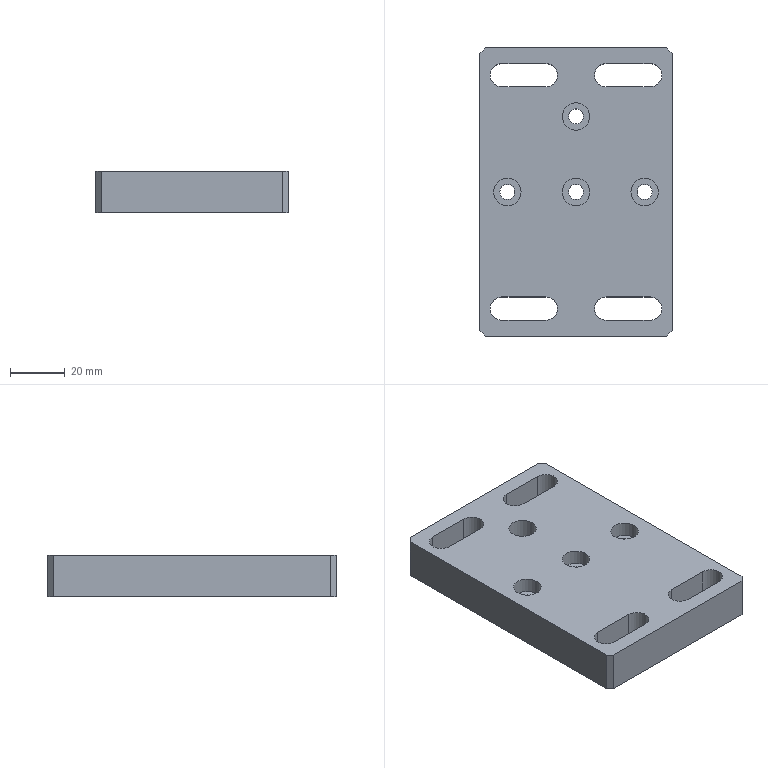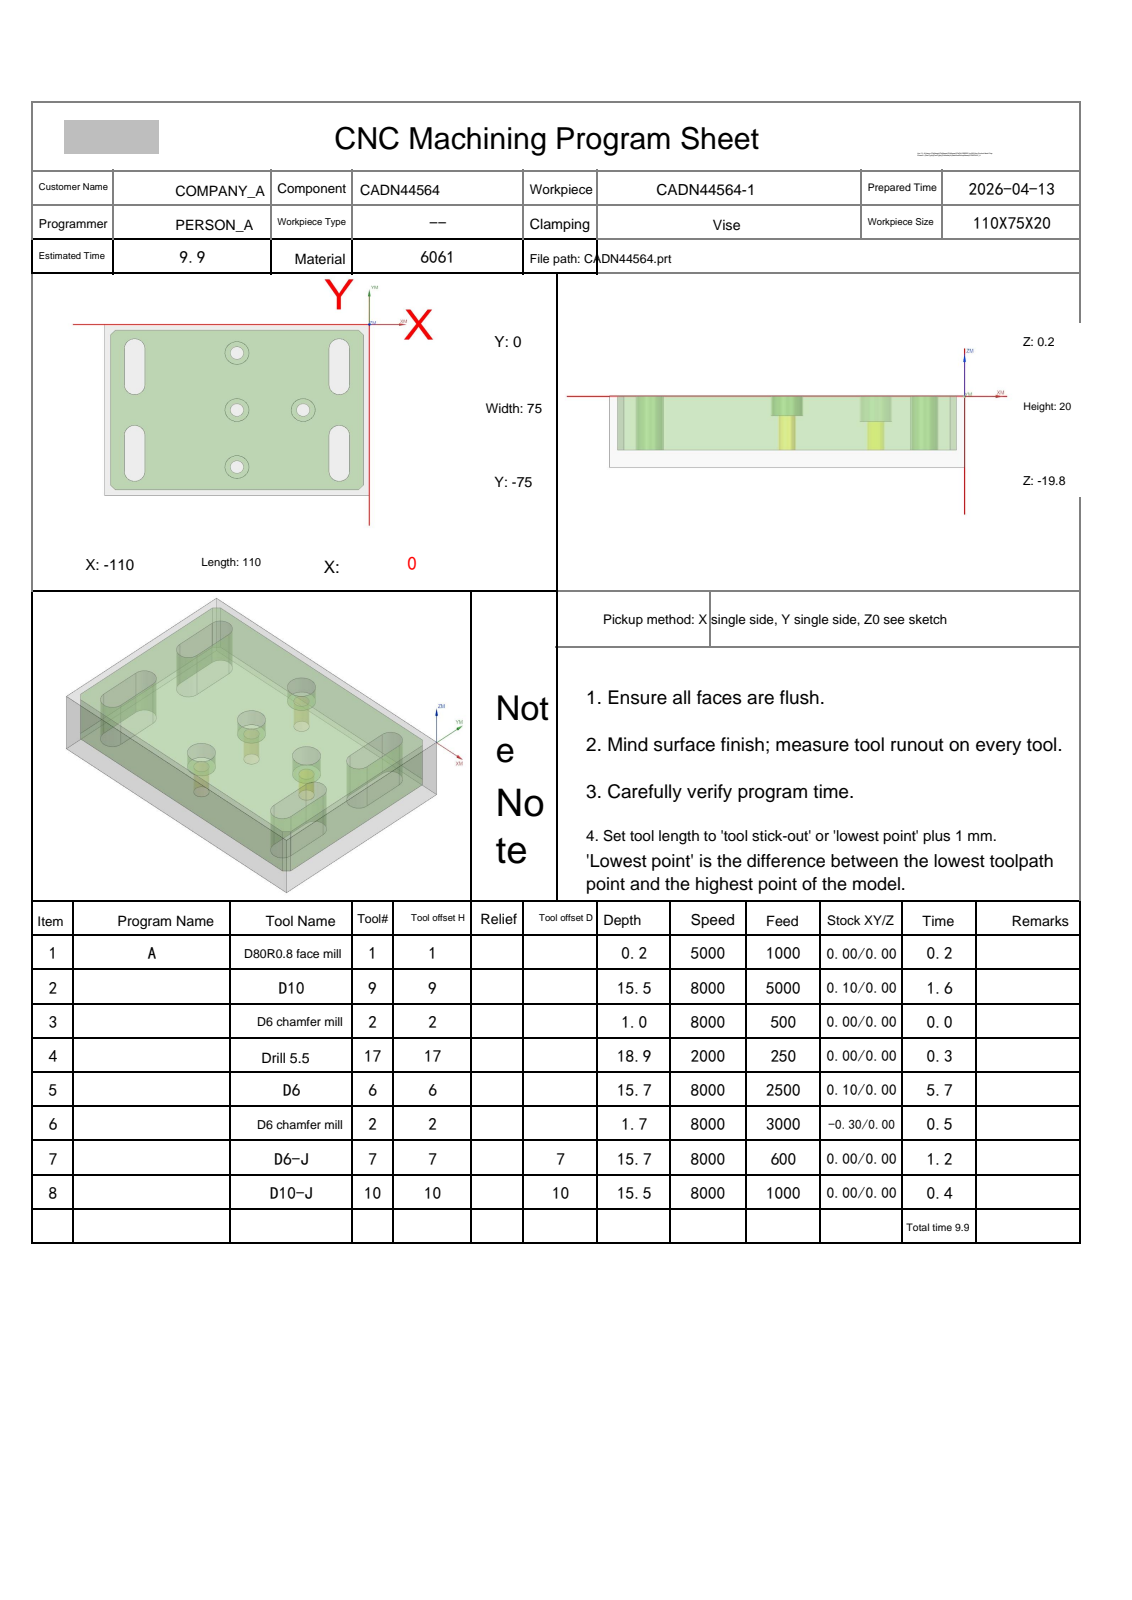NC program | NX | posted by the shop | part box 70 x 105 x 15 mm
Lines 418 to 1208 of 3183:
N5 T06 M06
(D6  D=6. R=0. H=06 ce=0.10 di=0.10)
G00 G90 G54 X-11.35 Y-18.5 M03 S6000
G43 H06 Z20.
M08
Z.5
G01 Y-10.5 Z.459 F2500.
G03 X-12.5 Y-9.35 Z.45 I-1.15 J0.0
X-13.65 Y-10.5 Z.441 I0.0 J-1.15
G01 Y-26.5 Z.359
G03 X-12.5 Y-27.65 Z.35 I1.15 J0.0
X-11.35 Y-26.5 Z.341 I0.0 J1.15
G01 Y-10.5 Z.259
G03 X-12.5 Y-9.35 Z.25 I-1.15 J0.0
X-13.65 Y-10.5 Z.241 I0.0 J-1.15
G01 Y-26.5 Z.159
G03 X-12.5 Y-27.65 Z.15 I1.15 J0.0
X-11.35 Y-26.5 Z.141 I0.0 J1.15
G01 Y-10.5 Z.059
G03 X-12.5 Y-9.35 Z.05 I-1.15 J0.0
X-13.65 Y-10.5 Z.041 I0.0 J-1.15
G01 Y-26.5 Z-.041
G03 X-12.5 Y-27.65 Z-.05 I1.15 J0.0
X-11.35 Y-26.5 Z-.059 I0.0 J1.15
G01 Y-10.5 Z-.141
G03 X-12.5 Y-9.35 Z-.15 I-1.15 J0.0
X-13.65 Y-10.5 Z-.159 I0.0 J-1.15
G01 Y-26.5 Z-.241
G03 X-12.5 Y-27.65 Z-.25 I1.15 J0.0
X-11.35 Y-26.5 Z-.259 I0.0 J1.15
G01 Y-10.5 Z-.341
G03 X-12.5 Y-9.35 Z-.35 I-1.15 J0.0
X-13.65 Y-10.5 Z-.359 I0.0 J-1.15
G01 Y-26.5 Z-.441
G03 X-12.5 Y-27.65 Z-.45 I1.15 J0.0
X-11.35 Y-26.5 Z-.459 I0.0 J1.15
G01 Y-10.5 Z-.541
G03 X-12.5 Y-9.35 Z-.55 I-1.15 J0.0
X-13.65 Y-10.5 Z-.559 I0.0 J-1.15
G01 Y-26.5 Z-.641
G03 X-12.5 Y-27.65 Z-.65 I1.15 J0.0
X-11.35 Y-26.5 Z-.659 I0.0 J1.15
G01 Y-10.5 Z-.741
G03 X-12.5 Y-9.35 Z-.75 I-1.15 J0.0
X-13.65 Y-10.5 Z-.759 I0.0 J-1.15
G01 Y-26.5 Z-.841
G03 X-12.5 Y-27.65 Z-.85 I1.15 J0.0
X-11.35 Y-26.5 Z-.859 I0.0 J1.15
G01 Y-10.5 Z-.941
G03 X-12.5 Y-9.35 Z-.95 I-1.15 J0.0
X-13.65 Y-10.5 Z-.959 I0.0 J-1.15
G01 Y-26.5 Z-1.041
G03 X-12.5 Y-27.65 Z-1.05 I1.15 J0.0
X-11.35 Y-26.5 Z-1.059 I0.0 J1.15
G01 Y-10.5 Z-1.141
G03 X-12.5 Y-9.35 Z-1.15 I-1.15 J0.0
X-13.65 Y-10.5 Z-1.159 I0.0 J-1.15
G01 Y-26.5 Z-1.241
G03 X-12.5 Y-27.65 Z-1.25 I1.15 J0.0
X-11.35 Y-26.5 Z-1.259 I0.0 J1.15
G01 Y-10.5 Z-1.341
G03 X-12.5 Y-9.35 Z-1.35 I-1.15 J0.0
X-13.65 Y-10.5 Z-1.359 I0.0 J-1.15
G01 Y-26.5 Z-1.441
G03 X-12.5 Y-27.65 Z-1.45 I1.15 J0.0
X-11.35 Y-26.5 Z-1.459 I0.0 J1.15
G01 Y-10.5 Z-1.541
G03 X-12.5 Y-9.35 Z-1.55 I-1.15 J0.0
X-13.65 Y-10.5 Z-1.559 I0.0 J-1.15
G01 Y-26.5 Z-1.641
G03 X-12.5 Y-27.65 Z-1.65 I1.15 J0.0
X-11.35 Y-26.5 Z-1.659 I0.0 J1.15
G01 Y-10.5 Z-1.741
G03 X-12.5 Y-9.35 Z-1.75 I-1.15 J0.0
X-13.65 Y-10.5 Z-1.759 I0.0 J-1.15
G01 Y-26.5 Z-1.841
G03 X-12.5 Y-27.65 Z-1.85 I1.15 J0.0
X-11.35 Y-26.5 Z-1.859 I0.0 J1.15
G01 Y-10.5 Z-1.941
G03 X-12.5 Y-9.35 Z-1.95 I-1.15 J0.0
X-13.65 Y-10.5 Z-1.959 I0.0 J-1.15
G01 Y-26.5 Z-2.041
G03 X-12.5 Y-27.65 Z-2.05 I1.15 J0.0
X-11.35 Y-26.5 Z-2.059 I0.0 J1.15
G01 Y-10.5 Z-2.141
G03 X-12.5 Y-9.35 Z-2.15 I-1.15 J0.0
X-13.65 Y-10.5 Z-2.159 I0.0 J-1.15
G01 Y-26.5 Z-2.241
G03 X-12.5 Y-27.65 Z-2.25 I1.15 J0.0
X-11.35 Y-26.5 Z-2.259 I0.0 J1.15
G01 Y-10.5 Z-2.341
G03 X-12.5 Y-9.35 Z-2.35 I-1.15 J0.0
X-13.65 Y-10.5 Z-2.359 I0.0 J-1.15
G01 Y-26.5 Z-2.441
G03 X-12.5 Y-27.65 Z-2.45 I1.15 J0.0
X-11.35 Y-26.5 Z-2.459 I0.0 J1.15
G01 Y-10.5 Z-2.541
G03 X-12.5 Y-9.35 Z-2.55 I-1.15 J0.0
X-13.65 Y-10.5 Z-2.559 I0.0 J-1.15
G01 Y-26.5 Z-2.641
G03 X-12.5 Y-27.65 Z-2.65 I1.15 J0.0
X-11.35 Y-26.5 Z-2.659 I0.0 J1.15
G01 Y-10.5 Z-2.741
G03 X-12.5 Y-9.35 Z-2.75 I-1.15 J0.0
X-13.65 Y-10.5 Z-2.759 I0.0 J-1.15
G01 Y-26.5 Z-2.841
G03 X-12.5 Y-27.65 Z-2.85 I1.15 J0.0
X-11.35 Y-26.5 Z-2.859 I0.0 J1.15
G01 Y-10.5 Z-2.941
G03 X-12.5 Y-9.35 Z-2.95 I-1.15 J0.0
X-13.65 Y-10.5 Z-2.959 I0.0 J-1.15
G01 Y-26.5 Z-3.041
G03 X-12.5 Y-27.65 Z-3.05 I1.15 J0.0
X-11.35 Y-26.5 Z-3.059 I0.0 J1.15
G01 Y-10.5 Z-3.141
G03 X-12.5 Y-9.35 Z-3.15 I-1.15 J0.0
X-13.65 Y-10.5 Z-3.159 I0.0 J-1.15
G01 Y-26.5 Z-3.241
G03 X-12.5 Y-27.65 Z-3.25 I1.15 J0.0
X-11.35 Y-26.5 Z-3.259 I0.0 J1.15
G01 Y-10.5 Z-3.341
G03 X-12.5 Y-9.35 Z-3.35 I-1.15 J0.0
X-13.65 Y-10.5 Z-3.359 I0.0 J-1.15
G01 Y-26.5 Z-3.441
G03 X-12.5 Y-27.65 Z-3.45 I1.15 J0.0
X-11.35 Y-26.5 Z-3.459 I0.0 J1.15
G01 Y-10.5 Z-3.541
G03 X-12.5 Y-9.35 Z-3.55 I-1.15 J0.0
X-13.65 Y-10.5 Z-3.559 I0.0 J-1.15
G01 Y-26.5 Z-3.641
G03 X-12.5 Y-27.65 Z-3.65 I1.15 J0.0
X-11.35 Y-26.5 Z-3.659 I0.0 J1.15
G01 Y-10.5 Z-3.741
G03 X-12.5 Y-9.35 Z-3.75 I-1.15 J0.0
X-13.65 Y-10.5 Z-3.759 I0.0 J-1.15
G01 Y-26.5 Z-3.841
G03 X-12.5 Y-27.65 Z-3.85 I1.15 J0.0
X-11.35 Y-26.5 Z-3.859 I0.0 J1.15
G01 Y-10.5 Z-3.941
G03 X-12.5 Y-9.35 Z-3.95 I-1.15 J0.0
X-13.65 Y-10.5 Z-3.959 I0.0 J-1.15
G01 Y-26.5 Z-4.041
G03 X-12.5 Y-27.65 Z-4.05 I1.15 J0.0
X-11.35 Y-26.5 Z-4.059 I0.0 J1.15
G01 Y-10.5 Z-4.141
G03 X-12.5 Y-9.35 Z-4.15 I-1.15 J0.0
X-13.65 Y-10.5 Z-4.159 I0.0 J-1.15
G01 Y-26.5 Z-4.241
G03 X-12.5 Y-27.65 Z-4.25 I1.15 J0.0
X-11.35 Y-26.5 Z-4.259 I0.0 J1.15
G01 Y-10.5 Z-4.341
G03 X-12.5 Y-9.35 Z-4.35 I-1.15 J0.0
X-13.65 Y-10.5 Z-4.359 I0.0 J-1.15
G01 Y-26.5 Z-4.441
G03 X-12.5 Y-27.65 Z-4.45 I1.15 J0.0
X-11.35 Y-26.5 Z-4.459 I0.0 J1.15
G01 Y-10.5 Z-4.541
G03 X-12.5 Y-9.35 Z-4.55 I-1.15 J0.0
X-13.65 Y-10.5 Z-4.559 I0.0 J-1.15
G01 Y-26.5 Z-4.641
G03 X-12.5 Y-27.65 Z-4.65 I1.15 J0.0
X-11.35 Y-26.5 Z-4.659 I0.0 J1.15
G01 Y-10.5 Z-4.741
G03 X-12.5 Y-9.35 Z-4.75 I-1.15 J0.0
X-13.65 Y-10.5 Z-4.759 I0.0 J-1.15
G01 Y-26.5 Z-4.841
G03 X-12.5 Y-27.65 Z-4.85 I1.15 J0.0
X-11.35 Y-26.5 Z-4.859 I0.0 J1.15
G01 Y-10.5 Z-4.941
G03 X-12.5 Y-9.35 Z-4.95 I-1.15 J0.0
X-13.65 Y-10.5 Z-4.959 I0.0 J-1.15
G01 Y-26.5 Z-5.041
G03 X-12.5 Y-27.65 Z-5.05 I1.15 J0.0
X-11.35 Y-26.5 Z-5.059 I0.0 J1.15
G01 Y-10.5 Z-5.141
G03 X-12.5 Y-9.35 Z-5.15 I-1.15 J0.0
X-13.65 Y-10.5 Z-5.159 I0.0 J-1.15
G01 Y-26.5 Z-5.241
G03 X-12.5 Y-27.65 Z-5.25 I1.15 J0.0
X-11.35 Y-26.5 Z-5.259 I0.0 J1.15
G01 Y-10.5 Z-5.341
G03 X-12.5 Y-9.35 Z-5.35 I-1.15 J0.0
X-13.65 Y-10.5 Z-5.359 I0.0 J-1.15
G01 Y-26.5 Z-5.441
G03 X-12.5 Y-27.65 Z-5.45 I1.15 J0.0
X-11.35 Y-26.5 Z-5.459 I0.0 J1.15
G01 Y-10.5 Z-5.541
G03 X-12.5 Y-9.35 Z-5.55 I-1.15 J0.0
X-13.65 Y-10.5 Z-5.559 I0.0 J-1.15
G01 Y-26.5 Z-5.641
G03 X-12.5 Y-27.65 Z-5.65 I1.15 J0.0
X-11.35 Y-26.5 Z-5.659 I0.0 J1.15
G01 Y-10.5 Z-5.741
G03 X-12.5 Y-9.35 Z-5.75 I-1.15 J0.0
X-13.65 Y-10.5 Z-5.759 I0.0 J-1.15
G01 Y-26.5 Z-5.841
G03 X-12.5 Y-27.65 Z-5.85 I1.15 J0.0
X-11.35 Y-26.5 Z-5.859 I0.0 J1.15
G01 Y-10.5 Z-5.941
G03 X-12.5 Y-9.35 Z-5.95 I-1.15 J0.0
X-13.65 Y-10.5 Z-5.959 I0.0 J-1.15
G01 Y-26.5 Z-6.041
G03 X-12.5 Y-27.65 Z-6.05 I1.15 J0.0
X-11.35 Y-26.5 Z-6.059 I0.0 J1.15
G01 Y-10.5 Z-6.141
G03 X-12.5 Y-9.35 Z-6.15 I-1.15 J0.0
X-13.65 Y-10.5 Z-6.159 I0.0 J-1.15
G01 Y-26.5 Z-6.241
G03 X-12.5 Y-27.65 Z-6.25 I1.15 J0.0
X-11.35 Y-26.5 Z-6.259 I0.0 J1.15
G01 Y-10.5 Z-6.341
G03 X-12.5 Y-9.35 Z-6.35 I-1.15 J0.0
X-13.65 Y-10.5 Z-6.359 I0.0 J-1.15
G01 Y-26.5 Z-6.441
G03 X-12.5 Y-27.65 Z-6.45 I1.15 J0.0
X-11.35 Y-26.5 Z-6.459 I0.0 J1.15
G01 Y-10.5 Z-6.541
G03 X-12.5 Y-9.35 Z-6.55 I-1.15 J0.0
X-13.65 Y-10.5 Z-6.559 I0.0 J-1.15
G01 Y-26.5 Z-6.641
G03 X-12.5 Y-27.65 Z-6.65 I1.15 J0.0
X-11.35 Y-26.5 Z-6.659 I0.0 J1.15
G01 Y-10.5 Z-6.741
G03 X-12.5 Y-9.35 Z-6.75 I-1.15 J0.0
X-13.65 Y-10.5 Z-6.759 I0.0 J-1.15
G01 Y-26.5 Z-6.841
G03 X-12.5 Y-27.65 Z-6.85 I1.15 J0.0
X-11.35 Y-26.5 Z-6.859 I0.0 J1.15
G01 Y-10.5 Z-6.941
G03 X-12.5 Y-9.35 Z-6.95 I-1.15 J0.0
X-13.65 Y-10.5 Z-6.959 I0.0 J-1.15
G01 Y-26.5 Z-7.041
G03 X-12.5 Y-27.65 Z-7.05 I1.15 J0.0
X-11.35 Y-26.5 Z-7.059 I0.0 J1.15
G01 Y-10.5 Z-7.141
G03 X-12.5 Y-9.35 Z-7.15 I-1.15 J0.0
X-13.65 Y-10.5 Z-7.159 I0.0 J-1.15
G01 Y-26.5 Z-7.241
G03 X-12.5 Y-27.65 Z-7.25 I1.15 J0.0
X-11.35 Y-26.5 Z-7.259 I0.0 J1.15
G01 Y-10.5 Z-7.341
G03 X-12.5 Y-9.35 Z-7.35 I-1.15 J0.0
X-13.65 Y-10.5 Z-7.359 I0.0 J-1.15
G01 Y-26.5 Z-7.441
G03 X-12.5 Y-27.65 Z-7.45 I1.15 J0.0
X-11.35 Y-26.5 Z-7.459 I0.0 J1.15
G01 Y-10.5 Z-7.541
G03 X-12.5 Y-9.35 Z-7.55 I-1.15 J0.0
X-13.65 Y-10.5 Z-7.559 I0.0 J-1.15
G01 Y-26.5 Z-7.641
G03 X-12.5 Y-27.65 Z-7.65 I1.15 J0.0
X-11.35 Y-26.5 Z-7.659 I0.0 J1.15
G01 Y-10.5 Z-7.741
G03 X-12.5 Y-9.35 Z-7.75 I-1.15 J0.0
X-13.65 Y-10.5 Z-7.759 I0.0 J-1.15
G01 Y-26.5 Z-7.841
G03 X-12.5 Y-27.65 Z-7.85 I1.15 J0.0
X-11.35 Y-26.5 Z-7.859 I0.0 J1.15
G01 Y-10.5 Z-7.941
G03 X-12.5 Y-9.35 Z-7.95 I-1.15 J0.0
X-13.65 Y-10.5 Z-7.959 I0.0 J-1.15
G01 Y-26.5 Z-8.041
G03 X-12.5 Y-27.65 Z-8.05 I1.15 J0.0
X-11.35 Y-26.5 Z-8.059 I0.0 J1.15
G01 Y-10.5 Z-8.141
G03 X-12.5 Y-9.35 Z-8.15 I-1.15 J0.0
X-13.65 Y-10.5 Z-8.159 I0.0 J-1.15
G01 Y-26.5 Z-8.241
G03 X-12.5 Y-27.65 Z-8.25 I1.15 J0.0
X-11.35 Y-26.5 Z-8.259 I0.0 J1.15
G01 Y-10.5 Z-8.341
G03 X-12.5 Y-9.35 Z-8.35 I-1.15 J0.0
X-13.65 Y-10.5 Z-8.359 I0.0 J-1.15
G01 Y-26.5 Z-8.441
G03 X-12.5 Y-27.65 Z-8.45 I1.15 J0.0
X-11.35 Y-26.5 Z-8.459 I0.0 J1.15
G01 Y-10.5 Z-8.541
G03 X-12.5 Y-9.35 Z-8.55 I-1.15 J0.0
X-13.65 Y-10.5 Z-8.559 I0.0 J-1.15
G01 Y-26.5 Z-8.641
G03 X-12.5 Y-27.65 Z-8.65 I1.15 J0.0
X-11.35 Y-26.5 Z-8.659 I0.0 J1.15
G01 Y-10.5 Z-8.741
G03 X-12.5 Y-9.35 Z-8.75 I-1.15 J0.0
X-13.65 Y-10.5 Z-8.759 I0.0 J-1.15
G01 Y-26.5 Z-8.841
G03 X-12.5 Y-27.65 Z-8.85 I1.15 J0.0
X-11.35 Y-26.5 Z-8.859 I0.0 J1.15
G01 Y-10.5 Z-8.941
G03 X-12.5 Y-9.35 Z-8.95 I-1.15 J0.0
X-13.65 Y-10.5 Z-8.959 I0.0 J-1.15
G01 Y-26.5 Z-9.041
G03 X-12.5 Y-27.65 Z-9.05 I1.15 J0.0
X-11.35 Y-26.5 Z-9.059 I0.0 J1.15
G01 Y-10.5 Z-9.141
G03 X-12.5 Y-9.35 Z-9.15 I-1.15 J0.0
X-13.65 Y-10.5 Z-9.159 I0.0 J-1.15
G01 Y-26.5 Z-9.241
G03 X-12.5 Y-27.65 Z-9.25 I1.15 J0.0
X-11.35 Y-26.5 Z-9.259 I0.0 J1.15
G01 Y-10.5 Z-9.341
G03 X-12.5 Y-9.35 Z-9.35 I-1.15 J0.0
X-13.65 Y-10.5 Z-9.359 I0.0 J-1.15
G01 Y-26.5 Z-9.441
G03 X-12.5 Y-27.65 Z-9.45 I1.15 J0.0
X-11.35 Y-26.5 Z-9.459 I0.0 J1.15
G01 Y-10.5 Z-9.541
G03 X-12.5 Y-9.35 Z-9.55 I-1.15 J0.0
X-13.65 Y-10.5 Z-9.559 I0.0 J-1.15
G01 Y-26.5 Z-9.641
G03 X-12.5 Y-27.65 Z-9.65 I1.15 J0.0
X-11.35 Y-26.5 Z-9.659 I0.0 J1.15
G01 Y-10.5 Z-9.741
G03 X-12.5 Y-9.35 Z-9.75 I-1.15 J0.0
X-13.65 Y-10.5 Z-9.759 I0.0 J-1.15
G01 Y-26.5 Z-9.841
G03 X-12.5 Y-27.65 Z-9.85 I1.15 J0.0
X-11.35 Y-26.5 Z-9.859 I0.0 J1.15
G01 Y-10.5 Z-9.941
G03 X-12.5 Y-9.35 Z-9.95 I-1.15 J0.0
X-13.65 Y-10.5 Z-9.959 I0.0 J-1.15
G01 Y-26.5 Z-10.041
G03 X-12.5 Y-27.65 Z-10.05 I1.15 J0.0
X-11.35 Y-26.5 Z-10.059 I0.0 J1.15
G01 Y-10.5 Z-10.141
G03 X-12.5 Y-9.35 Z-10.15 I-1.15 J0.0
X-13.65 Y-10.5 Z-10.159 I0.0 J-1.15
G01 Y-26.5 Z-10.241
G03 X-12.5 Y-27.65 Z-10.25 I1.15 J0.0
X-11.35 Y-26.5 Z-10.259 I0.0 J1.15
G01 Y-10.5 Z-10.341
G03 X-12.5 Y-9.35 Z-10.35 I-1.15 J0.0
X-13.65 Y-10.5 Z-10.359 I0.0 J-1.15
G01 Y-26.5 Z-10.441
G03 X-12.5 Y-27.65 Z-10.45 I1.15 J0.0
X-11.35 Y-26.5 Z-10.459 I0.0 J1.15
G01 Y-10.5 Z-10.541
G03 X-12.5 Y-9.35 Z-10.55 I-1.15 J0.0
X-13.65 Y-10.5 Z-10.559 I0.0 J-1.15
G01 Y-26.5 Z-10.641
G03 X-12.5 Y-27.65 Z-10.65 I1.15 J0.0
X-11.35 Y-26.5 Z-10.659 I0.0 J1.15
G01 Y-10.5 Z-10.741
G03 X-12.5 Y-9.35 Z-10.75 I-1.15 J0.0
X-13.65 Y-10.5 Z-10.759 I0.0 J-1.15
G01 Y-26.5 Z-10.841
G03 X-12.5 Y-27.65 Z-10.85 I1.15 J0.0
X-11.35 Y-26.5 Z-10.859 I0.0 J1.15
G01 Y-10.5 Z-10.941
G03 X-12.5 Y-9.35 Z-10.95 I-1.15 J0.0
X-13.65 Y-10.5 Z-10.959 I0.0 J-1.15
G01 Y-26.5 Z-11.041
G03 X-12.5 Y-27.65 Z-11.05 I1.15 J0.0
X-11.35 Y-26.5 Z-11.059 I0.0 J1.15
G01 Y-10.5 Z-11.141
G03 X-12.5 Y-9.35 Z-11.15 I-1.15 J0.0
X-13.65 Y-10.5 Z-11.159 I0.0 J-1.15
G01 Y-26.5 Z-11.241
G03 X-12.5 Y-27.65 Z-11.25 I1.15 J0.0
X-11.35 Y-26.5 Z-11.259 I0.0 J1.15
G01 Y-10.5 Z-11.341
G03 X-12.5 Y-9.35 Z-11.35 I-1.15 J0.0
X-13.65 Y-10.5 Z-11.359 I0.0 J-1.15
G01 Y-26.5 Z-11.441
G03 X-12.5 Y-27.65 Z-11.45 I1.15 J0.0
X-11.35 Y-26.5 Z-11.459 I0.0 J1.15
G01 Y-10.5 Z-11.541
G03 X-12.5 Y-9.35 Z-11.55 I-1.15 J0.0
X-13.65 Y-10.5 Z-11.559 I0.0 J-1.15
G01 Y-26.5 Z-11.641
G03 X-12.5 Y-27.65 Z-11.65 I1.15 J0.0
X-11.35 Y-26.5 Z-11.659 I0.0 J1.15
G01 Y-10.5 Z-11.741
G03 X-12.5 Y-9.35 Z-11.75 I-1.15 J0.0
X-13.65 Y-10.5 Z-11.759 I0.0 J-1.15
G01 Y-26.5 Z-11.841
G03 X-12.5 Y-27.65 Z-11.85 I1.15 J0.0
X-11.35 Y-26.5 Z-11.859 I0.0 J1.15
G01 Y-10.5 Z-11.941
G03 X-12.5 Y-9.35 Z-11.95 I-1.15 J0.0
X-13.65 Y-10.5 Z-11.959 I0.0 J-1.15
G01 Y-26.5 Z-12.041
G03 X-12.5 Y-27.65 Z-12.05 I1.15 J0.0
X-11.35 Y-26.5 Z-12.059 I0.0 J1.15
G01 Y-10.5 Z-12.141
G03 X-12.5 Y-9.35 Z-12.15 I-1.15 J0.0
X-13.65 Y-10.5 Z-12.159 I0.0 J-1.15
G01 Y-26.5 Z-12.241
G03 X-12.5 Y-27.65 Z-12.25 I1.15 J0.0
X-11.35 Y-26.5 Z-12.259 I0.0 J1.15
G01 Y-10.5 Z-12.341
G03 X-12.5 Y-9.35 Z-12.35 I-1.15 J0.0
X-13.65 Y-10.5 Z-12.359 I0.0 J-1.15
G01 Y-26.5 Z-12.441
G03 X-12.5 Y-27.65 Z-12.45 I1.15 J0.0
X-11.35 Y-26.5 Z-12.459 I0.0 J1.15
G01 Y-10.5 Z-12.541
G03 X-12.5 Y-9.35 Z-12.55 I-1.15 J0.0
X-13.65 Y-10.5 Z-12.559 I0.0 J-1.15
G01 Y-26.5 Z-12.641
G03 X-12.5 Y-27.65 Z-12.65 I1.15 J0.0
X-11.35 Y-26.5 Z-12.659 I0.0 J1.15
G01 Y-10.5 Z-12.741
G03 X-12.5 Y-9.35 Z-12.75 I-1.15 J0.0
X-13.65 Y-10.5 Z-12.759 I0.0 J-1.15
G01 Y-26.5 Z-12.841
G03 X-12.5 Y-27.65 Z-12.85 I1.15 J0.0
X-11.35 Y-26.5 Z-12.859 I0.0 J1.15
G01 Y-10.5 Z-12.941
G03 X-12.5 Y-9.35 Z-12.95 I-1.15 J0.0
X-13.65 Y-10.5 Z-12.959 I0.0 J-1.15
G01 Y-26.5 Z-13.041
G03 X-12.5 Y-27.65 Z-13.05 I1.15 J0.0
X-11.35 Y-26.5 Z-13.059 I0.0 J1.15
G01 Y-10.5 Z-13.141
G03 X-12.5 Y-9.35 Z-13.15 I-1.15 J0.0
X-13.65 Y-10.5 Z-13.159 I0.0 J-1.15
G01 Y-26.5 Z-13.241
G03 X-12.5 Y-27.65 Z-13.25 I1.15 J0.0
X-11.35 Y-26.5 Z-13.259 I0.0 J1.15
G01 Y-10.5 Z-13.341
G03 X-12.5 Y-9.35 Z-13.35 I-1.15 J0.0
X-13.65 Y-10.5 Z-13.359 I0.0 J-1.15
G01 Y-26.5 Z-13.441
G03 X-12.5 Y-27.65 Z-13.45 I1.15 J0.0
X-11.35 Y-26.5 Z-13.459 I0.0 J1.15
G01 Y-10.5 Z-13.541
G03 X-12.5 Y-9.35 Z-13.55 I-1.15 J0.0
X-13.65 Y-10.5 Z-13.559 I0.0 J-1.15
G01 Y-26.5 Z-13.641
G03 X-12.5 Y-27.65 Z-13.65 I1.15 J0.0
X-11.35 Y-26.5 Z-13.659 I0.0 J1.15
G01 Y-10.5 Z-13.741
G03 X-12.5 Y-9.35 Z-13.75 I-1.15 J0.0
X-13.65 Y-10.5 Z-13.759 I0.0 J-1.15
G01 Y-26.5 Z-13.841
G03 X-12.5 Y-27.65 Z-13.85 I1.15 J0.0
X-11.35 Y-26.5 Z-13.859 I0.0 J1.15
G01 Y-10.5 Z-13.941
G03 X-12.5 Y-9.35 Z-13.95 I-1.15 J0.0
X-13.65 Y-10.5 Z-13.959 I0.0 J-1.15
G01 Y-26.5 Z-14.041
G03 X-12.5 Y-27.65 Z-14.05 I1.15 J0.0
X-11.35 Y-26.5 Z-14.059 I0.0 J1.15
G01 Y-10.5 Z-14.141
G03 X-12.5 Y-9.35 Z-14.15 I-1.15 J0.0
X-13.65 Y-10.5 Z-14.159 I0.0 J-1.15
G01 Y-26.5 Z-14.241
G03 X-12.5 Y-27.65 Z-14.25 I1.15 J0.0
X-11.35 Y-26.5 Z-14.259 I0.0 J1.15
G01 Y-10.5 Z-14.341
G03 X-12.5 Y-9.35 Z-14.35 I-1.15 J0.0
X-13.65 Y-10.5 Z-14.359 I0.0 J-1.15
G01 Y-26.5 Z-14.441
G03 X-12.5 Y-27.65 Z-14.45 I1.15 J0.0
X-11.35 Y-26.5 Z-14.459 I0.0 J1.15
G01 Y-10.5 Z-14.541
G03 X-12.5 Y-9.35 Z-14.55 I-1.15 J0.0
X-13.65 Y-10.5 Z-14.559 I0.0 J-1.15
G01 Y-26.5 Z-14.641
G03 X-12.5 Y-27.65 Z-14.65 I1.15 J0.0
X-11.35 Y-26.5 Z-14.659 I0.0 J1.15
G01 Y-10.5 Z-14.741
G03 X-12.5 Y-9.35 Z-14.75 I-1.15 J0.0
X-13.65 Y-10.5 Z-14.759 I0.0 J-1.15
G01 Y-26.5 Z-14.841
G03 X-12.5 Y-27.65 Z-14.85 I1.15 J0.0
X-11.35 Y-26.5 Z-14.859 I0.0 J1.15
G01 Y-10.5 Z-14.941
G03 X-12.5 Y-9.35 Z-14.95 I-1.15 J0.0
X-13.65 Y-10.5 Z-14.959 I0.0 J-1.15
G01 Y-26.5 Z-15.041
G03 X-12.5 Y-27.65 Z-15.05 I1.15 J0.0
X-11.35 Y-26.5 Z-15.059 I0.0 J1.15
G01 Y-10.5 Z-15.141
G03 X-12.5 Y-9.35 Z-15.15 I-1.15 J0.0
X-13.65 Y-10.5 Z-15.159 I0.0 J-1.15
G01 Y-26.5 Z-15.241
G03 X-12.5 Y-27.65 Z-15.25 I1.15 J0.0
X-11.35 Y-26.5 Z-15.259 I0.0 J1.15
G01 Y-10.5 Z-15.341
G03 X-12.5 Y-9.35 Z-15.35 I-1.15 J0.0
X-13.65 Y-10.5 Z-15.359 I0.0 J-1.15
G01 Y-26.5 Z-15.441
G03 X-12.5 Y-27.65 Z-15.45 I1.15 J0.0
X-11.35 Y-26.5 Z-15.459 I0.0 J1.15
G01 Y-18.5 Z-15.5
Y-10.5
G03 X-12.5 Y-9.35 I-1.15 J0.0
X-13.65 Y-10.5 I0.0 J-1.15
G01 Y-26.5
G03 X-12.5 Y-27.65 I1.15 J0.0
X-11.35 Y-26.5 I0.0 J1.15
G01 Y-18.5
Y-18.
Z-14.5
G00 Z20.
Y-56.5
Z.5
G01 Y-48.5 Z.459
G03 X-12.5 Y-47.35 Z.45 I-1.15 J0.0
X-13.65 Y-48.5 Z.441 I0.0 J-1.15
G01 Y-64.5 Z.359
G03 X-13.142 Y-65.454 Z.353 I1.15 J0.0
X-12.5 Y-65.65 Z.35 I.642 J.954
X-11.35 Y-64.5 Z.341 I0.0 J1.15
G01 Y-48.5 Z.259
G03 X-12.5 Y-47.35 Z.25 I-1.15 J0.0
X-13.65 Y-48.5 Z.241 I0.0 J-1.15
G01 Y-64.5 Z.159
G03 X-13.142 Y-65.454 Z.153 I1.15 J0.0
X-12.5 Y-65.65 Z.15 I.642 J.954
X-11.35 Y-64.5 Z.141 I0.0 J1.15
G01 Y-48.5 Z.059
G03 X-12.5 Y-47.35 Z.05 I-1.15 J0.0
X-13.65 Y-48.5 Z.041 I0.0 J-1.15
G01 Y-64.5 Z-.041
G03 X-13.142 Y-65.454 Z-.047 I1.15 J0.0
X-12.5 Y-65.65 Z-.05 I.642 J.954
X-11.35 Y-64.5 Z-.059 I0.0 J1.15
G01 Y-48.5 Z-.141
G03 X-12.5 Y-47.35 Z-.15 I-1.15 J0.0
X-13.65 Y-48.5 Z-.159 I0.0 J-1.15
G01 Y-64.5 Z-.241
G03 X-13.142 Y-65.454 Z-.247 I1.15 J0.0
X-12.5 Y-65.65 Z-.25 I.642 J.954
X-11.35 Y-64.5 Z-.259 I0.0 J1.15
G01 Y-48.5 Z-.341
G03 X-12.5 Y-47.35 Z-.35 I-1.15 J0.0
X-13.65 Y-48.5 Z-.359 I0.0 J-1.15
G01 Y-64.5 Z-.441
G03 X-13.142 Y-65.454 Z-.447 I1.15 J0.0
X-12.5 Y-65.65 Z-.45 I.642 J.954
X-11.35 Y-64.5 Z-.459 I0.0 J1.15
G01 Y-48.5 Z-.541
G03 X-12.5 Y-47.35 Z-.55 I-1.15 J0.0
X-13.65 Y-48.5 Z-.559 I0.0 J-1.15
G01 Y-64.5 Z-.641
G03 X-13.142 Y-65.454 Z-.647 I1.15 J0.0
X-12.5 Y-65.65 Z-.65 I.642 J.954
X-11.35 Y-64.5 Z-.659 I0.0 J1.15
G01 Y-48.5 Z-.741
G03 X-12.5 Y-47.35 Z-.75 I-1.15 J0.0
X-13.65 Y-48.5 Z-.759 I0.0 J-1.15
G01 Y-64.5 Z-.841
G03 X-13.142 Y-65.454 Z-.847 I1.15 J0.0
X-12.5 Y-65.65 Z-.85 I.642 J.954
X-11.35 Y-64.5 Z-.859 I0.0 J1.15
G01 Y-48.5 Z-.941
G03 X-12.5 Y-47.35 Z-.95 I-1.15 J0.0
X-13.65 Y-48.5 Z-.959 I0.0 J-1.15
G01 Y-64.5 Z-1.041
G03 X-13.142 Y-65.454 Z-1.047 I1.15 J0.0
X-12.5 Y-65.65 Z-1.05 I.642 J.954
X-11.35 Y-64.5 Z-1.059 I0.0 J1.15
G01 Y-48.5 Z-1.141
G03 X-12.5 Y-47.35 Z-1.15 I-1.15 J0.0
X-13.65 Y-48.5 Z-1.159 I0.0 J-1.15
G01 Y-64.5 Z-1.241
G03 X-13.142 Y-65.454 Z-1.247 I1.15 J0.0
X-12.5 Y-65.65 Z-1.25 I.642 J.954
X-11.35 Y-64.5 Z-1.259 I0.0 J1.15
G01 Y-48.5 Z-1.341
G03 X-12.5 Y-47.35 Z-1.35 I-1.15 J0.0
X-13.65 Y-48.5 Z-1.359 I0.0 J-1.15
G01 Y-64.5 Z-1.441
G03 X-13.142 Y-65.454 Z-1.447 I1.15 J0.0
X-12.5 Y-65.65 Z-1.45 I.642 J.954
X-11.35 Y-64.5 Z-1.459 I0.0 J1.15
G01 Y-48.5 Z-1.541
G03 X-12.5 Y-47.35 Z-1.55 I-1.15 J0.0
X-13.65 Y-48.5 Z-1.559 I0.0 J-1.15
G01 Y-64.5 Z-1.641
G03 X-13.142 Y-65.454 Z-1.647 I1.15 J0.0
X-12.5 Y-65.65 Z-1.65 I.642 J.954
X-11.35 Y-64.5 Z-1.659 I0.0 J1.15
G01 Y-48.5 Z-1.741
G03 X-12.5 Y-47.35 Z-1.75 I-1.15 J0.0
X-13.65 Y-48.5 Z-1.759 I0.0 J-1.15
G01 Y-64.5 Z-1.841
G03 X-13.142 Y-65.454 Z-1.847 I1.15 J0.0
X-12.5 Y-65.65 Z-1.85 I.642 J.954
X-11.35 Y-64.5 Z-1.859 I0.0 J1.15
G01 Y-48.5 Z-1.941
G03 X-12.5 Y-47.35 Z-1.95 I-1.15 J0.0
X-13.65 Y-48.5 Z-1.959 I0.0 J-1.15
G01 Y-64.5 Z-2.041
G03 X-13.142 Y-65.454 Z-2.047 I1.15 J0.0
X-12.5 Y-65.65 Z-2.05 I.642 J.954
X-11.35 Y-64.5 Z-2.059 I0.0 J1.15
G01 Y-48.5 Z-2.141
G03 X-12.5 Y-47.35 Z-2.15 I-1.15 J0.0
X-13.65 Y-48.5 Z-2.159 I0.0 J-1.15
G01 Y-64.5 Z-2.241
G03 X-13.142 Y-65.454 Z-2.247 I1.15 J0.0
X-12.5 Y-65.65 Z-2.25 I.642 J.954
X-11.35 Y-64.5 Z-2.259 I0.0 J1.15
G01 Y-48.5 Z-2.341
G03 X-12.5 Y-47.35 Z-2.35 I-1.15 J0.0
X-13.65 Y-48.5 Z-2.359 I0.0 J-1.15
G01 Y-64.5 Z-2.441
G03 X-13.142 Y-65.454 Z-2.447 I1.15 J0.0
X-12.5 Y-65.65 Z-2.45 I.642 J.954
X-11.35 Y-64.5 Z-2.459 I0.0 J1.15
G01 Y-48.5 Z-2.541
G03 X-12.5 Y-47.35 Z-2.55 I-1.15 J0.0
X-13.65 Y-48.5 Z-2.559 I0.0 J-1.15
G01 Y-64.5 Z-2.641
G03 X-13.142 Y-65.454 Z-2.647 I1.15 J0.0
X-12.5 Y-65.65 Z-2.65 I.642 J.954
X-11.35 Y-64.5 Z-2.659 I0.0 J1.15
G01 Y-48.5 Z-2.741
G03 X-12.5 Y-47.35 Z-2.75 I-1.15 J0.0
X-13.65 Y-48.5 Z-2.759 I0.0 J-1.15
G01 Y-64.5 Z-2.841
G03 X-13.142 Y-65.454 Z-2.847 I1.15 J0.0
X-12.5 Y-65.65 Z-2.85 I.642 J.954
X-11.35 Y-64.5 Z-2.859 I0.0 J1.15
G01 Y-48.5 Z-2.941
G03 X-12.5 Y-47.35 Z-2.95 I-1.15 J0.0
X-13.65 Y-48.5 Z-2.959 I0.0 J-1.15
G01 Y-64.5 Z-3.041
G03 X-13.142 Y-65.454 Z-3.047 I1.15 J0.0
X-12.5 Y-65.65 Z-3.05 I.642 J.954
X-11.35 Y-64.5 Z-3.059 I0.0 J1.15
G01 Y-48.5 Z-3.141
G03 X-12.5 Y-47.35 Z-3.15 I-1.15 J0.0
X-13.65 Y-48.5 Z-3.159 I0.0 J-1.15
G01 Y-64.5 Z-3.241
G03 X-13.142 Y-65.454 Z-3.247 I1.15 J0.0
X-12.5 Y-65.65 Z-3.25 I.642 J.954
X-11.35 Y-64.5 Z-3.259 I0.0 J1.15
G01 Y-48.5 Z-3.341
G03 X-12.5 Y-47.35 Z-3.35 I-1.15 J0.0
X-13.65 Y-48.5 Z-3.359 I0.0 J-1.15
G01 Y-64.5 Z-3.441
G03 X-13.142 Y-65.454 Z-3.447 I1.15 J0.0
X-12.5 Y-65.65 Z-3.45 I.642 J.954
X-11.35 Y-64.5 Z-3.459 I0.0 J1.15
G01 Y-48.5 Z-3.541
G03 X-12.5 Y-47.35 Z-3.55 I-1.15 J0.0
X-13.65 Y-48.5 Z-3.559 I0.0 J-1.15
G01 Y-64.5 Z-3.641
G03 X-13.142 Y-65.454 Z-3.647 I1.15 J0.0
X-12.5 Y-65.65 Z-3.65 I.642 J.954
X-11.35 Y-64.5 Z-3.659 I0.0 J1.15
G01 Y-48.5 Z-3.741
G03 X-12.5 Y-47.35 Z-3.75 I-1.15 J0.0
X-13.65 Y-48.5 Z-3.759 I0.0 J-1.15
G01 Y-64.5 Z-3.841
G03 X-13.142 Y-65.454 Z-3.847 I1.15 J0.0
X-12.5 Y-65.65 Z-3.85 I.642 J.954
X-11.35 Y-64.5 Z-3.859 I0.0 J1.15
G01 Y-48.5 Z-3.941
G03 X-12.5 Y-47.35 Z-3.95 I-1.15 J0.0
X-13.65 Y-48.5 Z-3.959 I0.0 J-1.15
G01 Y-64.5 Z-4.041
G03 X-13.142 Y-65.454 Z-4.047 I1.15 J0.0
X-12.5 Y-65.65 Z-4.05 I.642 J.954
X-11.35 Y-64.5 Z-4.059 I0.0 J1.15
G01 Y-48.5 Z-4.141
G03 X-12.5 Y-47.35 Z-4.15 I-1.15 J0.0
X-13.65 Y-48.5 Z-4.159 I0.0 J-1.15
G01 Y-64.5 Z-4.241
G03 X-13.142 Y-65.454 Z-4.247 I1.15 J0.0
X-12.5 Y-65.65 Z-4.25 I.642 J.954
X-11.35 Y-64.5 Z-4.259 I0.0 J1.15
G01 Y-48.5 Z-4.341
G03 X-12.5 Y-47.35 Z-4.35 I-1.15 J0.0
X-13.65 Y-48.5 Z-4.359 I0.0 J-1.15
G01 Y-64.5 Z-4.441
G03 X-13.142 Y-65.454 Z-4.447 I1.15 J0.0
X-12.5 Y-65.65 Z-4.45 I.642 J.954
X-11.35 Y-64.5 Z-4.459 I0.0 J1.15
G01 Y-48.5 Z-4.541
G03 X-12.5 Y-47.35 Z-4.55 I-1.15 J0.0
X-13.65 Y-48.5 Z-4.559 I0.0 J-1.15
G01 Y-64.5 Z-4.641
G03 X-13.142 Y-65.454 Z-4.647 I1.15 J0.0
X-12.5 Y-65.65 Z-4.65 I.642 J.954
X-11.35 Y-64.5 Z-4.659 I0.0 J1.15
G01 Y-48.5 Z-4.741
G03 X-12.5 Y-47.35 Z-4.75 I-1.15 J0.0
X-13.65 Y-48.5 Z-4.759 I0.0 J-1.15
G01 Y-64.5 Z-4.841
G03 X-13.142 Y-65.454 Z-4.847 I1.15 J0.0
X-12.5 Y-65.65 Z-4.85 I.642 J.954
X-11.35 Y-64.5 Z-4.859 I0.0 J1.15
G01 Y-48.5 Z-4.941
G03 X-12.5 Y-47.35 Z-4.95 I-1.15 J0.0
X-13.65 Y-48.5 Z-4.959 I0.0 J-1.15
G01 Y-64.5 Z-5.041
G03 X-13.142 Y-65.454 Z-5.047 I1.15 J0.0
X-12.5 Y-65.65 Z-5.05 I.642 J.954
X-11.35 Y-64.5 Z-5.059 I0.0 J1.15
G01 Y-48.5 Z-5.141
G03 X-12.5 Y-47.35 Z-5.15 I-1.15 J0.0
X-13.65 Y-48.5 Z-5.159 I0.0 J-1.15
G01 Y-64.5 Z-5.241
G03 X-13.142 Y-65.454 Z-5.247 I1.15 J0.0
X-12.5 Y-65.65 Z-5.25 I.642 J.954
X-11.35 Y-64.5 Z-5.259 I0.0 J1.15
G01 Y-48.5 Z-5.341
G03 X-12.5 Y-47.35 Z-5.35 I-1.15 J0.0
X-13.65 Y-48.5 Z-5.359 I0.0 J-1.15
G01 Y-64.5 Z-5.441
G03 X-13.142 Y-65.454 Z-5.447 I1.15 J0.0
X-12.5 Y-65.65 Z-5.45 I.642 J.954
X-11.35 Y-64.5 Z-5.459 I0.0 J1.15
G01 Y-48.5 Z-5.541
G03 X-12.5 Y-47.35 Z-5.55 I-1.15 J0.0
X-13.65 Y-48.5 Z-5.559 I0.0 J-1.15
G01 Y-64.5 Z-5.641
G03 X-13.142 Y-65.454 Z-5.647 I1.15 J0.0
X-12.5 Y-65.65 Z-5.65 I.642 J.954
X-11.35 Y-64.5 Z-5.659 I0.0 J1.15
G01 Y-48.5 Z-5.741
G03 X-12.5 Y-47.35 Z-5.75 I-1.15 J0.0
X-13.65 Y-48.5 Z-5.759 I0.0 J-1.15
G01 Y-64.5 Z-5.841
G03 X-13.142 Y-65.454 Z-5.847 I1.15 J0.0
X-12.5 Y-65.65 Z-5.85 I.642 J.954
X-11.35 Y-64.5 Z-5.859 I0.0 J1.15
G01 Y-48.5 Z-5.941
G03 X-12.5 Y-47.35 Z-5.95 I-1.15 J0.0
X-13.65 Y-48.5 Z-5.959 I0.0 J-1.15
G01 Y-64.5 Z-6.041
G03 X-13.142 Y-65.454 Z-6.047 I1.15 J0.0
X-12.5 Y-65.65 Z-6.05 I.642 J.954
X-11.35 Y-64.5 Z-6.059 I0.0 J1.15
G01 Y-48.5 Z-6.141
G03 X-12.5 Y-47.35 Z-6.15 I-1.15 J0.0
X-13.65 Y-48.5 Z-6.159 I0.0 J-1.15
G01 Y-64.5 Z-6.241
G03 X-13.142 Y-65.454 Z-6.247 I1.15 J0.0
X-12.5 Y-65.65 Z-6.25 I.642 J.954
X-11.35 Y-64.5 Z-6.259 I0.0 J1.15
G01 Y-48.5 Z-6.341
G03 X-12.5 Y-47.35 Z-6.35 I-1.15 J0.0
X-13.65 Y-48.5 Z-6.359 I0.0 J-1.15
G01 Y-64.5 Z-6.441
G03 X-13.142 Y-65.454 Z-6.447 I1.15 J0.0
X-12.5 Y-65.65 Z-6.45 I.642 J.954
X-11.35 Y-64.5 Z-6.459 I0.0 J1.15
G01 Y-48.5 Z-6.541
G03 X-12.5 Y-47.35 Z-6.55 I-1.15 J0.0
X-13.65 Y-48.5 Z-6.559 I0.0 J-1.15
G01 Y-64.5 Z-6.641
G03 X-13.142 Y-65.454 Z-6.647 I1.15 J0.0
X-12.5 Y-65.65 Z-6.65 I.642 J.954
X-11.35 Y-64.5 Z-6.659 I0.0 J1.15
G01 Y-48.5 Z-6.741
G03 X-12.5 Y-47.35 Z-6.75 I-1.15 J0.0
X-13.65 Y-48.5 Z-6.759 I0.0 J-1.15
G01 Y-64.5 Z-6.841
G03 X-13.142 Y-65.454 Z-6.847 I1.15 J0.0
X-12.5 Y-65.65 Z-6.85 I.642 J.954
X-11.35 Y-64.5 Z-6.859 I0.0 J1.15
G01 Y-48.5 Z-6.941
G03 X-12.5 Y-47.35 Z-6.95 I-1.15 J0.0
X-13.65 Y-48.5 Z-6.959 I0.0 J-1.15
G01 Y-64.5 Z-7.041
G03 X-13.142 Y-65.454 Z-7.047 I1.15 J0.0
X-12.5 Y-65.65 Z-7.05 I.642 J.954
X-11.35 Y-64.5 Z-7.059 I0.0 J1.15
G01 Y-48.5 Z-7.141
G03 X-12.5 Y-47.35 Z-7.15 I-1.15 J0.0
X-13.65 Y-48.5 Z-7.159 I0.0 J-1.15
G01 Y-64.5 Z-7.241
G03 X-13.142 Y-65.454 Z-7.247 I1.15 J0.0
X-12.5 Y-65.65 Z-7.25 I.642 J.954
X-11.35 Y-64.5 Z-7.259 I0.0 J1.15
G01 Y-48.5 Z-7.341
G03 X-12.5 Y-47.35 Z-7.35 I-1.15 J0.0
X-13.65 Y-48.5 Z-7.359 I0.0 J-1.15
G01 Y-64.5 Z-7.441
G03 X-13.142 Y-65.454 Z-7.447 I1.15 J0.0
X-12.5 Y-65.65 Z-7.45 I.642 J.954
X-11.35 Y-64.5 Z-7.459 I0.0 J1.15
G01 Y-48.5 Z-7.541
G03 X-12.5 Y-47.35 Z-7.55 I-1.15 J0.0
X-13.65 Y-48.5 Z-7.559 I0.0 J-1.15
G01 Y-64.5 Z-7.641
G03 X-13.142 Y-65.454 Z-7.647 I1.15 J0.0
X-12.5 Y-65.65 Z-7.65 I.642 J.954
X-11.35 Y-64.5 Z-7.659 I0.0 J1.15
G01 Y-48.5 Z-7.741
G03 X-12.5 Y-47.35 Z-7.75 I-1.15 J0.0
X-13.65 Y-48.5 Z-7.759 I0.0 J-1.15
G01 Y-64.5 Z-7.841
G03 X-13.142 Y-65.454 Z-7.847 I1.15 J0.0